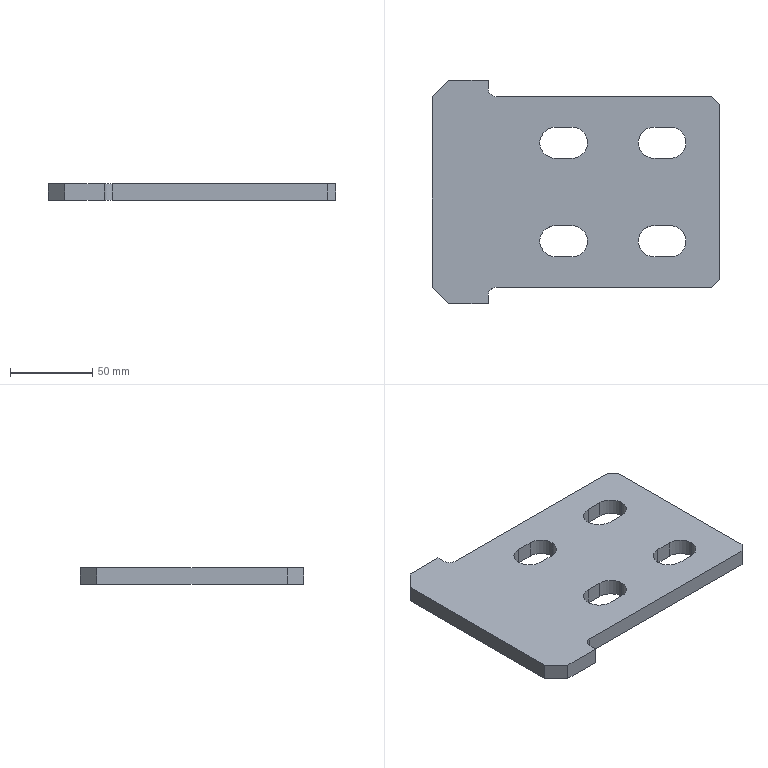Part | STEP file | 筋Plate-150×75-150-60度 | 1 solid | 36 faces | box 175 x 136 x 10 mm | volume 189716 mm3 | plane 22 | cylinder 14 | commonest cylinder face diameters 19 x12 10 x2